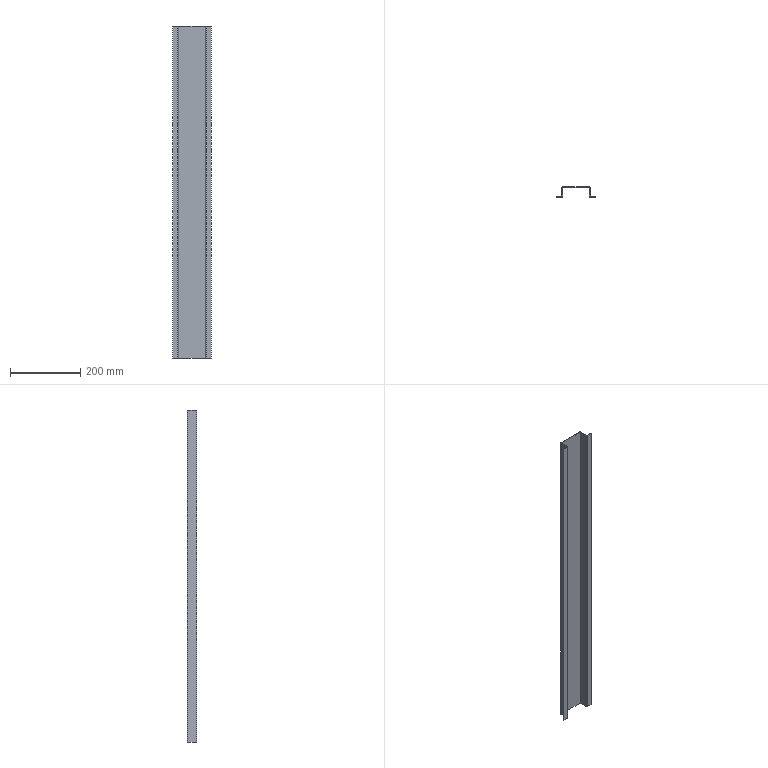Part | SolidWorks | features FlatPattern 1, SMBaseFlange 1, SheetMetal 1 | 1 solid | 38 faces | box 110 x 28.5 x 948 mm | volume 230156 mm3 | plane 30 | cylinder 8 | commonest cylinder face diameters 1 x4 4 x4
STEP:
#1=CARTESIAN_POINT('',(-40.,0.5,474.));
#2=VERTEX_POINT('',#1);
#3=CARTESIAN_POINT('',(-38.5,0.5,474.));
#4=VERTEX_POINT('',#3);
#5=CARTESIAN_POINT('',(-40.,0.5,474.));
#6=DIRECTION('',(1.,0.,0.));
#7=VECTOR('',#6,1000.);
#8=LINE('',#5,#7);
#9=EDGE_CURVE('',#2,#4,#8,.T.);
#10=ORIENTED_EDGE('',*,*,#9,.F.);
#11=CARTESIAN_POINT('',(-40.5,0.,474.));
#12=VERTEX_POINT('',#11);
#13=CARTESIAN_POINT('',(-40.5,0.5,474.));
#14=DIRECTION('',(0.,0.,-1.));
#15=DIRECTION('',(-1.,0.,0.));
#16=AXIS2_PLACEMENT_3D('',#13,#14,#15);
#17=CIRCLE('',#16,0.5);
#18=EDGE_CURVE('',#2,#12,#17,.T.);
#19=ORIENTED_EDGE('',*,*,#18,.T.);
#20=CARTESIAN_POINT('',(-40.5,-1.5,474.));
#21=VERTEX_POINT('',#20);
#22=CARTESIAN_POINT('',(-40.5,-1.5,474.));
#23=DIRECTION('',(0.,1.,0.));
#24=VECTOR('',#23,1000.);
#25=LINE('',#22,#24);
#26=EDGE_CURVE('',#21,#12,#25,.T.);
#27=ORIENTED_EDGE('',*,*,#26,.F.);
#28=CARTESIAN_POINT('',(-40.5,0.5,474.));
#29=DIRECTION('',(0.,0.,-1.));
#30=DIRECTION('',(1.,0.,0.));
#31=AXIS2_PLACEMENT_3D('',#28,#29,#30);
#32=CIRCLE('',#31,2.);
#33=EDGE_CURVE('',#4,#21,#32,.T.);
#34=ORIENTED_EDGE('',*,*,#33,.F.);
#35=EDGE_LOOP('',(#10,#19,#27,#34));
#36=FACE_OUTER_BOUND('',#35,.T.);
#37=CARTESIAN_POINT('',(-40.,0.5,474.));
#38=DIRECTION('',(0.,0.,1.));
#39=DIRECTION('',(1.,0.,0.));
#40=AXIS2_PLACEMENT_3D('',#37,#38,#39);
#41=PLANE('',#40);
#42=ADVANCED_FACE('',(#36),#41,.T.);
#43=CARTESIAN_POINT('',(-40.,25.,474.));
#44=VERTEX_POINT('',#43);
#45=CARTESIAN_POINT('',(-40.,0.,474.));
#46=DIRECTION('',(0.,-1.,0.));
#47=VECTOR('',#46,1000.);
#48=LINE('',#45,#47);
#49=EDGE_CURVE('',#44,#2,#48,.T.);
#50=ORIENTED_EDGE('',*,*,#49,.T.);
#51=ORIENTED_EDGE('',*,*,#9,.T.);
#52=CARTESIAN_POINT('',(-38.5,25.,474.));
#53=VERTEX_POINT('',#52);
#54=CARTESIAN_POINT('',(-38.5,0.,474.));
#55=DIRECTION('',(0.,-1.,0.));
#56=VECTOR('',#55,1000.);
#57=LINE('',#54,#56);
#58=EDGE_CURVE('',#53,#4,#57,.T.);
#59=ORIENTED_EDGE('',*,*,#58,.F.);
#60=CARTESIAN_POINT('',(-38.5,25.,474.));
#61=DIRECTION('',(-1.,0.,0.));
#62=VECTOR('',#61,1000.);
#63=LINE('',#60,#62);
#64=EDGE_CURVE('',#53,#44,#63,.T.);
#65=ORIENTED_EDGE('',*,*,#64,.T.);
#66=EDGE_LOOP('',(#50,#51,#59,#65));
#67=FACE_OUTER_BOUND('',#66,.T.);
#68=CARTESIAN_POINT('',(-40.5,-1.5,474.));
#69=DIRECTION('',(0.,0.,1.));
#70=DIRECTION('',(1.,0.,0.));
#71=AXIS2_PLACEMENT_3D('',#68,#69,#70);
#72=PLANE('',#71);
#73=ADVANCED_FACE('',(#67),#72,.T.);
#74=CARTESIAN_POINT('',(-40.5,0.,-474.));
#75=VERTEX_POINT('',#74);
#76=CARTESIAN_POINT('',(-40.5,-1.5,-474.));
#77=VERTEX_POINT('',#76);
#78=CARTESIAN_POINT('',(-40.5,0.,-474.));
#79=DIRECTION('',(0.,-1.,0.));
#80=VECTOR('',#79,1000.);
#81=LINE('',#78,#80);
#82=EDGE_CURVE('',#75,#77,#81,.T.);
#83=ORIENTED_EDGE('',*,*,#82,.F.);
#84=CARTESIAN_POINT('',(-40.,0.5,-474.));
#85=VERTEX_POINT('',#84);
#86=CARTESIAN_POINT('',(-40.5,0.5,-474.));
#87=DIRECTION('',(0.,0.,-1.));
#88=DIRECTION('',(-1.,0.,0.));
#89=AXIS2_PLACEMENT_3D('',#86,#87,#88);
#90=CIRCLE('',#89,0.5);
#91=EDGE_CURVE('',#85,#75,#90,.T.);
#92=ORIENTED_EDGE('',*,*,#91,.F.);
#93=CARTESIAN_POINT('',(-38.5,0.5,-474.));
#94=VERTEX_POINT('',#93);
#95=CARTESIAN_POINT('',(-38.5,0.5,-474.));
#96=DIRECTION('',(-1.,0.,0.));
#97=VECTOR('',#96,1000.);
#98=LINE('',#95,#97);
#99=EDGE_CURVE('',#94,#85,#98,.T.);
#100=ORIENTED_EDGE('',*,*,#99,.F.);
#101=CARTESIAN_POINT('',(-40.5,0.5,-474.));
#102=DIRECTION('',(0.,0.,-1.));
#103=DIRECTION('',(1.,0.,0.));
#104=AXIS2_PLACEMENT_3D('',#101,#102,#103);
#105=CIRCLE('',#104,2.);
#106=EDGE_CURVE('',#94,#77,#105,.T.);
#107=ORIENTED_EDGE('',*,*,#106,.T.);
#108=EDGE_LOOP('',(#83,#92,#100,#107));
#109=FACE_OUTER_BOUND('',#108,.T.);
#110=CARTESIAN_POINT('',(-40.5,0.,-474.));
#111=DIRECTION('',(0.,0.,-1.));
#112=DIRECTION('',(-1.,0.,0.));
#113=AXIS2_PLACEMENT_3D('',#110,#111,#112);
#114=PLANE('',#113);
#115=ADVANCED_FACE('',(#109),#114,.T.);
#116=CARTESIAN_POINT('',(-55.,0.,-474.));
#117=VERTEX_POINT('',#116);
#118=CARTESIAN_POINT('',(-55.,0.,-474.));
#119=DIRECTION('',(-1.,0.,0.));
#120=VECTOR('',#119,1000.);
#121=LINE('',#118,#120);
#122=EDGE_CURVE('',#75,#117,#121,.T.);
#123=ORIENTED_EDGE('',*,*,#122,.F.);
#124=ORIENTED_EDGE('',*,*,#82,.T.);
#125=CARTESIAN_POINT('',(-55.,-1.5,-474.));
#126=VERTEX_POINT('',#125);
#127=CARTESIAN_POINT('',(-55.,-1.5,-474.));
#128=DIRECTION('',(-1.,0.,0.));
#129=VECTOR('',#128,1000.);
#130=LINE('',#127,#129);
#131=EDGE_CURVE('',#77,#126,#130,.T.);
#132=ORIENTED_EDGE('',*,*,#131,.T.);
#133=CARTESIAN_POINT('',(-55.,-1.5,-474.));
#134=DIRECTION('',(0.,1.,0.));
#135=VECTOR('',#134,1000.);
#136=LINE('',#133,#135);
#137=EDGE_CURVE('',#126,#117,#136,.T.);
#138=ORIENTED_EDGE('',*,*,#137,.T.);
#139=EDGE_LOOP('',(#123,#124,#132,#138));
#140=FACE_OUTER_BOUND('',#139,.T.);
#141=CARTESIAN_POINT('',(-38.5,0.5,-474.));
#142=DIRECTION('',(0.,0.,-1.));
#143=DIRECTION('',(-1.,0.,0.));
#144=AXIS2_PLACEMENT_3D('',#141,#142,#143);
#145=PLANE('',#144);
#146=ADVANCED_FACE('',(#140),#145,.T.);
#147=CARTESIAN_POINT('',(-38.,27.,474.));
#148=VERTEX_POINT('',#147);
#149=CARTESIAN_POINT('',(-38.,25.5,474.));
#150=VERTEX_POINT('',#149);
#151=CARTESIAN_POINT('',(-38.,27.,474.));
#152=DIRECTION('',(0.,-1.,0.));
#153=VECTOR('',#152,1000.);
#154=LINE('',#151,#153);
#155=EDGE_CURVE('',#148,#150,#154,.T.);
#156=ORIENTED_EDGE('',*,*,#155,.F.);
#157=CARTESIAN_POINT('',(-38.,25.,474.));
#158=DIRECTION('',(0.,0.,1.));
#159=DIRECTION('',(1.,0.,0.));
#160=AXIS2_PLACEMENT_3D('',#157,#158,#159);
#161=CIRCLE('',#160,2.);
#162=EDGE_CURVE('',#148,#44,#161,.T.);
#163=ORIENTED_EDGE('',*,*,#162,.T.);
#164=ORIENTED_EDGE('',*,*,#64,.F.);
#165=CARTESIAN_POINT('',(-38.,25.,474.));
#166=DIRECTION('',(0.,0.,1.));
#167=DIRECTION('',(1.,0.,0.));
#168=AXIS2_PLACEMENT_3D('',#165,#166,#167);
#169=CIRCLE('',#168,0.5);
#170=EDGE_CURVE('',#150,#53,#169,.T.);
#171=ORIENTED_EDGE('',*,*,#170,.F.);
#172=EDGE_LOOP('',(#156,#163,#164,#171));
#173=FACE_OUTER_BOUND('',#172,.T.);
#174=CARTESIAN_POINT('',(-38.,27.,474.));
#175=DIRECTION('',(0.,0.,1.));
#176=DIRECTION('',(1.,0.,0.));
#177=AXIS2_PLACEMENT_3D('',#174,#175,#176);
#178=PLANE('',#177);
#179=ADVANCED_FACE('',(#173),#178,.T.);
#180=CARTESIAN_POINT('',(38.,27.,474.));
#181=VERTEX_POINT('',#180);
#182=CARTESIAN_POINT('',(-40.,27.,474.));
#183=DIRECTION('',(-1.,0.,0.));
#184=VECTOR('',#183,1000.);
#185=LINE('',#182,#184);
#186=EDGE_CURVE('',#181,#148,#185,.T.);
#187=ORIENTED_EDGE('',*,*,#186,.T.);
#188=ORIENTED_EDGE('',*,*,#155,.T.);
#189=CARTESIAN_POINT('',(38.,25.5,474.));
#190=VERTEX_POINT('',#189);
#191=CARTESIAN_POINT('',(-40.,25.5,474.));
#192=DIRECTION('',(-1.,0.,0.));
#193=VECTOR('',#192,1000.);
#194=LINE('',#191,#193);
#195=EDGE_CURVE('',#190,#150,#194,.T.);
#196=ORIENTED_EDGE('',*,*,#195,.F.);
#197=CARTESIAN_POINT('',(38.,25.5,474.));
#198=DIRECTION('',(0.,1.,0.));
#199=VECTOR('',#198,1000.);
#200=LINE('',#197,#199);
#201=EDGE_CURVE('',#190,#181,#200,.T.);
#202=ORIENTED_EDGE('',*,*,#201,.T.);
#203=EDGE_LOOP('',(#187,#188,#196,#202));
#204=FACE_OUTER_BOUND('',#203,.T.);
#205=CARTESIAN_POINT('',(-38.5,25.,474.));
#206=DIRECTION('',(0.,0.,1.));
#207=DIRECTION('',(1.,0.,0.));
#208=AXIS2_PLACEMENT_3D('',#205,#206,#207);
#209=PLANE('',#208);
#210=ADVANCED_FACE('',(#204),#209,.T.);
#211=CARTESIAN_POINT('',(-40.,25.,-474.));
#212=VERTEX_POINT('',#211);
#213=CARTESIAN_POINT('',(-38.5,25.,-474.));
#214=VERTEX_POINT('',#213);
#215=CARTESIAN_POINT('',(-40.,25.,-474.));
#216=DIRECTION('',(1.,0.,0.));
#217=VECTOR('',#216,1000.);
#218=LINE('',#215,#217);
#219=EDGE_CURVE('',#212,#214,#218,.T.);
#220=ORIENTED_EDGE('',*,*,#219,.F.);
#221=CARTESIAN_POINT('',(-38.,27.,-474.));
#222=VERTEX_POINT('',#221);
#223=CARTESIAN_POINT('',(-38.,25.,-474.));
#224=DIRECTION('',(0.,0.,1.));
#225=DIRECTION('',(1.,0.,0.));
#226=AXIS2_PLACEMENT_3D('',#223,#224,#225);
#227=CIRCLE('',#226,2.);
#228=EDGE_CURVE('',#222,#212,#227,.T.);
#229=ORIENTED_EDGE('',*,*,#228,.F.);
#230=CARTESIAN_POINT('',(-38.,25.5,-474.));
#231=VERTEX_POINT('',#230);
#232=CARTESIAN_POINT('',(-38.,25.5,-474.));
#233=DIRECTION('',(0.,1.,0.));
#234=VECTOR('',#233,1000.);
#235=LINE('',#232,#234);
#236=EDGE_CURVE('',#231,#222,#235,.T.);
#237=ORIENTED_EDGE('',*,*,#236,.F.);
#238=CARTESIAN_POINT('',(-38.,25.,-474.));
#239=DIRECTION('',(0.,0.,1.));
#240=DIRECTION('',(1.,0.,0.));
#241=AXIS2_PLACEMENT_3D('',#238,#239,#240);
#242=CIRCLE('',#241,0.5);
#243=EDGE_CURVE('',#231,#214,#242,.T.);
#244=ORIENTED_EDGE('',*,*,#243,.T.);
#245=EDGE_LOOP('',(#220,#229,#237,#244));
#246=FACE_OUTER_BOUND('',#245,.T.);
#247=CARTESIAN_POINT('',(-40.,25.,-474.));
#248=DIRECTION('',(0.,0.,-1.));
#249=DIRECTION('',(-1.,0.,0.));
#250=AXIS2_PLACEMENT_3D('',#247,#248,#249);
#251=PLANE('',#250);
#252=ADVANCED_FACE('',(#246),#251,.T.);
#253=CARTESIAN_POINT('',(-40.,0.,-474.));
#254=DIRECTION('',(0.,-1.,0.));
#255=VECTOR('',#254,1000.);
#256=LINE('',#253,#255);
#257=EDGE_CURVE('',#212,#85,#256,.T.);
#258=ORIENTED_EDGE('',*,*,#257,.F.);
#259=ORIENTED_EDGE('',*,*,#219,.T.);
#260=CARTESIAN_POINT('',(-38.5,0.,-474.));
#261=DIRECTION('',(0.,-1.,0.));
#262=VECTOR('',#261,1000.);
#263=LINE('',#260,#262);
#264=EDGE_CURVE('',#214,#94,#263,.T.);
#265=ORIENTED_EDGE('',*,*,#264,.T.);
#266=ORIENTED_EDGE('',*,*,#99,.T.);
#267=EDGE_LOOP('',(#258,#259,#265,#266));
#268=FACE_OUTER_BOUND('',#267,.T.);
#269=CARTESIAN_POINT('',(-38.,25.5,-474.));
#270=DIRECTION('',(0.,0.,-1.));
#271=DIRECTION('',(-1.,0.,0.));
#272=AXIS2_PLACEMENT_3D('',#269,#270,#271);
#273=PLANE('',#272);
#274=ADVANCED_FACE('',(#268),#273,.T.);
#275=CARTESIAN_POINT('',(40.,25.,474.));
#276=VERTEX_POINT('',#275);
#277=CARTESIAN_POINT('',(38.5,25.,474.));
#278=VERTEX_POINT('',#277);
#279=CARTESIAN_POINT('',(40.,25.,474.));
#280=DIRECTION('',(-1.,0.,0.));
#281=VECTOR('',#280,1000.);
#282=LINE('',#279,#281);
#283=EDGE_CURVE('',#276,#278,#282,.T.);
#284=ORIENTED_EDGE('',*,*,#283,.F.);
#285=CARTESIAN_POINT('',(38.,25.,474.));
#286=DIRECTION('',(0.,0.,1.));
#287=DIRECTION('',(1.,0.,0.));
#288=AXIS2_PLACEMENT_3D('',#285,#286,#287);
#289=CIRCLE('',#288,2.);
#290=EDGE_CURVE('',#276,#181,#289,.T.);
#291=ORIENTED_EDGE('',*,*,#290,.T.);
#292=ORIENTED_EDGE('',*,*,#201,.F.);
#293=CARTESIAN_POINT('',(38.,25.,474.));
#294=DIRECTION('',(0.,0.,1.));
#295=DIRECTION('',(1.,0.,0.));
#296=AXIS2_PLACEMENT_3D('',#293,#294,#295);
#297=CIRCLE('',#296,0.5);
#298=EDGE_CURVE('',#278,#190,#297,.T.);
#299=ORIENTED_EDGE('',*,*,#298,.F.);
#300=EDGE_LOOP('',(#284,#291,#292,#299));
#301=FACE_OUTER_BOUND('',#300,.T.);
#302=CARTESIAN_POINT('',(40.,25.,474.));
#303=DIRECTION('',(0.,0.,1.));
#304=DIRECTION('',(1.,0.,0.));
#305=AXIS2_PLACEMENT_3D('',#302,#303,#304);
#306=PLANE('',#305);
#307=ADVANCED_FACE('',(#301),#306,.T.);
#308=CARTESIAN_POINT('',(40.,0.5,474.));
#309=VERTEX_POINT('',#308);
#310=CARTESIAN_POINT('',(40.,0.,474.));
#311=DIRECTION('',(0.,1.,0.));
#312=VECTOR('',#311,1000.);
#313=LINE('',#310,#312);
#314=EDGE_CURVE('',#309,#276,#313,.T.);
#315=ORIENTED_EDGE('',*,*,#314,.T.);
#316=ORIENTED_EDGE('',*,*,#283,.T.);
#317=CARTESIAN_POINT('',(38.5,0.5,474.));
#318=VERTEX_POINT('',#317);
#319=CARTESIAN_POINT('',(38.5,0.,474.));
#320=DIRECTION('',(0.,1.,0.));
#321=VECTOR('',#320,1000.);
#322=LINE('',#319,#321);
#323=EDGE_CURVE('',#318,#278,#322,.T.);
#324=ORIENTED_EDGE('',*,*,#323,.F.);
#325=CARTESIAN_POINT('',(38.5,0.5,474.));
#326=DIRECTION('',(1.,0.,0.));
#327=VECTOR('',#326,1000.);
#328=LINE('',#325,#327);
#329=EDGE_CURVE('',#318,#309,#328,.T.);
#330=ORIENTED_EDGE('',*,*,#329,.T.);
#331=EDGE_LOOP('',(#315,#316,#324,#330));
#332=FACE_OUTER_BOUND('',#331,.T.);
#333=CARTESIAN_POINT('',(38.,25.5,474.));
#334=DIRECTION('',(0.,0.,1.));
#335=DIRECTION('',(1.,0.,0.));
#336=AXIS2_PLACEMENT_3D('',#333,#334,#335);
#337=PLANE('',#336);
#338=ADVANCED_FACE('',(#332),#337,.T.);
#339=CARTESIAN_POINT('',(38.,27.,-474.));
#340=VERTEX_POINT('',#339);
#341=CARTESIAN_POINT('',(38.,25.5,-474.));
#342=VERTEX_POINT('',#341);
#343=CARTESIAN_POINT('',(38.,27.,-474.));
#344=DIRECTION('',(0.,-1.,0.));
#345=VECTOR('',#344,1000.);
#346=LINE('',#343,#345);
#347=EDGE_CURVE('',#340,#342,#346,.T.);
#348=ORIENTED_EDGE('',*,*,#347,.F.);
#349=CARTESIAN_POINT('',(40.,25.,-474.));
#350=VERTEX_POINT('',#349);
#351=CARTESIAN_POINT('',(38.,25.,-474.));
#352=DIRECTION('',(0.,0.,1.));
#353=DIRECTION('',(1.,0.,0.));
#354=AXIS2_PLACEMENT_3D('',#351,#352,#353);
#355=CIRCLE('',#354,2.);
#356=EDGE_CURVE('',#350,#340,#355,.T.);
#357=ORIENTED_EDGE('',*,*,#356,.F.);
#358=CARTESIAN_POINT('',(38.5,25.,-474.));
#359=VERTEX_POINT('',#358);
#360=CARTESIAN_POINT('',(38.5,25.,-474.));
#361=DIRECTION('',(1.,0.,0.));
#362=VECTOR('',#361,1000.);
#363=LINE('',#360,#362);
#364=EDGE_CURVE('',#359,#350,#363,.T.);
#365=ORIENTED_EDGE('',*,*,#364,.F.);
#366=CARTESIAN_POINT('',(38.,25.,-474.));
#367=DIRECTION('',(0.,0.,1.));
#368=DIRECTION('',(1.,0.,0.));
#369=AXIS2_PLACEMENT_3D('',#366,#367,#368);
#370=CIRCLE('',#369,0.5);
#371=EDGE_CURVE('',#359,#342,#370,.T.);
#372=ORIENTED_EDGE('',*,*,#371,.T.);
#373=EDGE_LOOP('',(#348,#357,#365,#372));
#374=FACE_OUTER_BOUND('',#373,.T.);
#375=CARTESIAN_POINT('',(38.,27.,-474.));
#376=DIRECTION('',(0.,0.,-1.));
#377=DIRECTION('',(-1.,0.,0.));
#378=AXIS2_PLACEMENT_3D('',#375,#376,#377);
#379=PLANE('',#378);
#380=ADVANCED_FACE('',(#374),#379,.T.);
#381=CARTESIAN_POINT('',(-40.,27.,-474.));
#382=DIRECTION('',(-1.,0.,0.));
#383=VECTOR('',#382,1000.);
#384=LINE('',#381,#383);
#385=EDGE_CURVE('',#340,#222,#384,.T.);
#386=ORIENTED_EDGE('',*,*,#385,.F.);
#387=ORIENTED_EDGE('',*,*,#347,.T.);
#388=CARTESIAN_POINT('',(-40.,25.5,-474.));
#389=DIRECTION('',(-1.,0.,0.));
#390=VECTOR('',#389,1000.);
#391=LINE('',#388,#390);
#392=EDGE_CURVE('',#342,#231,#391,.T.);
#393=ORIENTED_EDGE('',*,*,#392,.T.);
#394=ORIENTED_EDGE('',*,*,#236,.T.);
#395=EDGE_LOOP('',(#386,#387,#393,#394));
#396=FACE_OUTER_BOUND('',#395,.T.);
#397=CARTESIAN_POINT('',(38.5,25.,-474.));
#398=DIRECTION('',(0.,0.,-1.));
#399=DIRECTION('',(-1.,0.,0.));
#400=AXIS2_PLACEMENT_3D('',#397,#398,#399);
#401=PLANE('',#400);
#402=ADVANCED_FACE('',(#396),#401,.T.);
#403=CARTESIAN_POINT('',(40.5,0.,474.));
#404=VERTEX_POINT('',#403);
#405=CARTESIAN_POINT('',(40.5,-1.5,474.));
#406=VERTEX_POINT('',#405);
#407=CARTESIAN_POINT('',(40.5,0.,474.));
#408=DIRECTION('',(0.,-1.,0.));
#409=VECTOR('',#408,1000.);
#410=LINE('',#407,#409);
#411=EDGE_CURVE('',#404,#406,#410,.T.);
#412=ORIENTED_EDGE('',*,*,#411,.F.);
#413=CARTESIAN_POINT('',(40.5,0.5,474.));
#414=DIRECTION('',(0.,0.,-1.));
#415=DIRECTION('',(-1.,0.,0.));
#416=AXIS2_PLACEMENT_3D('',#413,#414,#415);
#417=CIRCLE('',#416,0.5);
#418=EDGE_CURVE('',#404,#309,#417,.T.);
#419=ORIENTED_EDGE('',*,*,#418,.T.);
#420=ORIENTED_EDGE('',*,*,#329,.F.);
#421=CARTESIAN_POINT('',(40.5,0.5,474.));
#422=DIRECTION('',(0.,0.,-1.));
#423=DIRECTION('',(1.,0.,0.));
#424=AXIS2_PLACEMENT_3D('',#421,#422,#423);
#425=CIRCLE('',#424,2.);
#426=EDGE_CURVE('',#406,#318,#425,.T.);
#427=ORIENTED_EDGE('',*,*,#426,.F.);
#428=EDGE_LOOP('',(#412,#419,#420,#427));
#429=FACE_OUTER_BOUND('',#428,.T.);
#430=CARTESIAN_POINT('',(40.5,0.,474.));
#431=DIRECTION('',(0.,0.,1.));
#432=DIRECTION('',(1.,0.,0.));
#433=AXIS2_PLACEMENT_3D('',#430,#431,#432);
#434=PLANE('',#433);
#435=ADVANCED_FACE('',(#429),#434,.T.);
#436=CARTESIAN_POINT('',(55.,0.,474.));
#437=VERTEX_POINT('',#436);
#438=CARTESIAN_POINT('',(55.,0.,474.));
#439=DIRECTION('',(-1.,0.,0.));
#440=VECTOR('',#439,1000.);
#441=LINE('',#438,#440);
#442=EDGE_CURVE('',#437,#404,#441,.T.);
#443=ORIENTED_EDGE('',*,*,#442,.T.);
#444=ORIENTED_EDGE('',*,*,#411,.T.);
#445=CARTESIAN_POINT('',(55.,-1.5,474.));
#446=VERTEX_POINT('',#445);
#447=CARTESIAN_POINT('',(55.,-1.5,474.));
#448=DIRECTION('',(-1.,0.,0.));
#449=VECTOR('',#448,1000.);
#450=LINE('',#447,#449);
#451=EDGE_CURVE('',#446,#406,#450,.T.);
#452=ORIENTED_EDGE('',*,*,#451,.F.);
#453=CARTESIAN_POINT('',(55.,0.,474.));
#454=DIRECTION('',(0.,-1.,0.));
#455=VECTOR('',#454,1000.);
#456=LINE('',#453,#455);
#457=EDGE_CURVE('',#437,#446,#456,.T.);
#458=ORIENTED_EDGE('',*,*,#457,.F.);
#459=EDGE_LOOP('',(#443,#444,#452,#458));
#460=FACE_OUTER_BOUND('',#459,.T.);
#461=CARTESIAN_POINT('',(38.5,0.5,474.));
#462=DIRECTION('',(0.,0.,1.));
#463=DIRECTION('',(1.,0.,0.));
#464=AXIS2_PLACEMENT_3D('',#461,#462,#463);
#465=PLANE('',#464);
#466=ADVANCED_FACE('',(#460),#465,.T.);
#467=CARTESIAN_POINT('',(40.,0.5,-474.));
#468=VERTEX_POINT('',#467);
#469=CARTESIAN_POINT('',(38.5,0.5,-474.));
#470=VERTEX_POINT('',#469);
#471=CARTESIAN_POINT('',(40.,0.5,-474.));
#472=DIRECTION('',(-1.,0.,0.));
#473=VECTOR('',#472,1000.);
#474=LINE('',#471,#473);
#475=EDGE_CURVE('',#468,#470,#474,.T.);
#476=ORIENTED_EDGE('',*,*,#475,.F.);
#477=CARTESIAN_POINT('',(40.5,0.,-474.));
#478=VERTEX_POINT('',#477);
#479=CARTESIAN_POINT('',(40.5,0.5,-474.));
#480=DIRECTION('',(0.,0.,-1.));
#481=DIRECTION('',(-1.,0.,0.));
#482=AXIS2_PLACEMENT_3D('',#479,#480,#481);
#483=CIRCLE('',#482,0.5);
#484=EDGE_CURVE('',#478,#468,#483,.T.);
#485=ORIENTED_EDGE('',*,*,#484,.F.);
#486=CARTESIAN_POINT('',(40.5,-1.5,-474.));
#487=VERTEX_POINT('',#486);
#488=CARTESIAN_POINT('',(40.5,-1.5,-474.));
#489=DIRECTION('',(0.,1.,0.));
#490=VECTOR('',#489,1000.);
#491=LINE('',#488,#490);
#492=EDGE_CURVE('',#487,#478,#491,.T.);
#493=ORIENTED_EDGE('',*,*,#492,.F.);
#494=CARTESIAN_POINT('',(40.5,0.5,-474.));
#495=DIRECTION('',(0.,0.,-1.));
#496=DIRECTION('',(1.,0.,0.));
#497=AXIS2_PLACEMENT_3D('',#494,#495,#496);
#498=CIRCLE('',#497,2.);
#499=EDGE_CURVE('',#487,#470,#498,.T.);
#500=ORIENTED_EDGE('',*,*,#499,.T.);
#501=EDGE_LOOP('',(#476,#485,#493,#500));
#502=FACE_OUTER_BOUND('',#501,.T.);
#503=CARTESIAN_POINT('',(40.,0.5,-474.));
#504=DIRECTION('',(0.,0.,-1.));
#505=DIRECTION('',(-1.,0.,0.));
#506=AXIS2_PLACEMENT_3D('',#503,#504,#505);
#507=PLANE('',#506);
#508=ADVANCED_FACE('',(#502),#507,.T.);
#509=CARTESIAN_POINT('',(40.,0.,-474.));
#510=DIRECTION('',(0.,1.,0.));
#511=VECTOR('',#510,1000.);
#512=LINE('',#509,#511);
#513=EDGE_CURVE('',#468,#350,#512,.T.);
#514=ORIENTED_EDGE('',*,*,#513,.F.);
#515=ORIENTED_EDGE('',*,*,#475,.T.);
#516=CARTESIAN_POINT('',(38.5,0.,-474.));
#517=DIRECTION('',(0.,1.,0.));
#518=VECTOR('',#517,1000.);
#519=LINE('',#516,#518);
#520=EDGE_CURVE('',#470,#359,#519,.T.);
#521=ORIENTED_EDGE('',*,*,#520,.T.);
#522=ORIENTED_EDGE('',*,*,#364,.T.);
#523=EDGE_LOOP('',(#514,#515,#521,#522));
#524=FACE_OUTER_BOUND('',#523,.T.);
#525=CARTESIAN_POINT('',(40.5,-1.5,-474.));
#526=DIRECTION('',(0.,0.,-1.));
#527=DIRECTION('',(-1.,0.,0.));
#528=AXIS2_PLACEMENT_3D('',#525,#526,#527);
#529=PLANE('',#528);
#530=ADVANCED_FACE('',(#524),#529,.T.);
#531=ORIENTED_EDGE('',*,*,#122,.T.);
#532=CARTESIAN_POINT('',(-55.,0.,474.));
#533=VERTEX_POINT('',#532);
#534=CARTESIAN_POINT('',(-55.,0.,474.));
#535=DIRECTION('',(0.,0.,-1.));
#536=VECTOR('',#535,1000.);
#537=LINE('',#534,#536);
#538=EDGE_CURVE('',#533,#117,#537,.T.);
#539=ORIENTED_EDGE('',*,*,#538,.F.);
#540=CARTESIAN_POINT('',(-55.,0.,474.));
#541=DIRECTION('',(-1.,0.,0.));
#542=VECTOR('',#541,1000.);
#543=LINE('',#540,#542);
#544=EDGE_CURVE('',#12,#533,#543,.T.);
#545=ORIENTED_EDGE('',*,*,#544,.F.);
#546=CARTESIAN_POINT('',(-40.5,0.,474.));
#547=DIRECTION('',(0.,0.,-1.));
#548=VECTOR('',#547,1000.);
#549=LINE('',#546,#548);
#550=EDGE_CURVE('',#12,#75,#549,.T.);
#551=ORIENTED_EDGE('',*,*,#550,.T.);
#552=EDGE_LOOP('',(#531,#539,#545,#551));
#553=FACE_OUTER_BOUND('',#552,.T.);
#554=CARTESIAN_POINT('',(-55.,0.,474.));
#555=DIRECTION('',(0.,-1.,0.));
#556=DIRECTION('',(0.,0.,-1.));
#557=AXIS2_PLACEMENT_3D('',#554,#555,#556);
#558=PLANE('',#557);
#559=ADVANCED_FACE('',(#553),#558,.F.);
#560=ORIENTED_EDGE('',*,*,#137,.F.);
#561=CARTESIAN_POINT('',(-55.,-1.5,474.));
#562=VERTEX_POINT('',#561);
#563=CARTESIAN_POINT('',(-55.,-1.5,474.));
#564=DIRECTION('',(0.,0.,-1.));
#565=VECTOR('',#564,1000.);
#566=LINE('',#563,#565);
#567=EDGE_CURVE('',#562,#126,#566,.T.);
#568=ORIENTED_EDGE('',*,*,#567,.F.);
#569=CARTESIAN_POINT('',(-55.,-1.5,474.));
#570=DIRECTION('',(0.,1.,0.));
#571=VECTOR('',#570,1000.);
#572=LINE('',#569,#571);
#573=EDGE_CURVE('',#562,#533,#572,.T.);
#574=ORIENTED_EDGE('',*,*,#573,.T.);
#575=ORIENTED_EDGE('',*,*,#538,.T.);
#576=EDGE_LOOP('',(#560,#568,#574,#575));
#577=FACE_OUTER_BOUND('',#576,.T.);
#578=CARTESIAN_POINT('',(-55.,-1.5,474.));
#579=DIRECTION('',(-1.,0.,0.));
#580=DIRECTION('',(0.,0.,1.));
#581=AXIS2_PLACEMENT_3D('',#578,#579,#580);
#582=PLANE('',#581);
#583=ADVANCED_FACE('',(#577),#582,.T.);
#584=ORIENTED_EDGE('',*,*,#131,.F.);
#585=CARTESIAN_POINT('',(-40.5,-1.5,474.));
#586=DIRECTION('',(0.,0.,-1.));
#587=VECTOR('',#586,1000.);
#588=LINE('',#585,#587);
#589=EDGE_CURVE('',#21,#77,#588,.T.);
#590=ORIENTED_EDGE('',*,*,#589,.F.);
#591=CARTESIAN_POINT('',(-55.,-1.5,474.));
#592=DIRECTION('',(-1.,0.,0.));
#593=VECTOR('',#592,1000.);
#594=LINE('',#591,#593);
#595=EDGE_CURVE('',#21,#562,#594,.T.);
#596=ORIENTED_EDGE('',*,*,#595,.T.);
#597=ORIENTED_EDGE('',*,*,#567,.T.);
#598=EDGE_LOOP('',(#584,#590,#596,#597));
#599=FACE_OUTER_BOUND('',#598,.T.);
#600=CARTESIAN_POINT('',(-55.,-1.5,474.));
#601=DIRECTION('',(0.,-1.,0.));
#602=DIRECTION('',(0.,0.,-1.));
#603=AXIS2_PLACEMENT_3D('',#600,#601,#602);
#604=PLANE('',#603);
#605=ADVANCED_FACE('',(#599),#604,.T.);
#606=ORIENTED_EDGE('',*,*,#106,.F.);
#607=CARTESIAN_POINT('',(-38.5,0.5,474.));
#608=DIRECTION('',(0.,0.,-1.));
#609=VECTOR('',#608,1000.);
#610=LINE('',#607,#609);
#611=EDGE_CURVE('',#4,#94,#610,.T.);
#612=ORIENTED_EDGE('',*,*,#611,.F.);
#613=ORIENTED_EDGE('',*,*,#33,.T.);
#614=ORIENTED_EDGE('',*,*,#589,.T.);
#615=EDGE_LOOP('',(#606,#612,#613,#614));
#616=FACE_OUTER_BOUND('',#615,.T.);
#617=CARTESIAN_POINT('',(-40.5,0.5,474.));
#618=DIRECTION('',(0.,0.,-1.));
#619=DIRECTION('',(-1.,0.,0.));
#620=AXIS2_PLACEMENT_3D('',#617,#618,#619);
#621=CYLINDRICAL_SURFACE('',#620,2.);
#622=ADVANCED_FACE('',(#616),#621,.T.);
#623=ORIENTED_EDGE('',*,*,#264,.F.);
#624=CARTESIAN_POINT('',(-38.5,25.,474.));
#625=DIRECTION('',(0.,0.,-1.));
#626=VECTOR('',#625,1000.);
#627=LINE('',#624,#626);
#628=EDGE_CURVE('',#53,#214,#627,.T.);
#629=ORIENTED_EDGE('',*,*,#628,.F.);
#630=ORIENTED_EDGE('',*,*,#58,.T.);
#631=ORIENTED_EDGE('',*,*,#611,.T.);
#632=EDGE_LOOP('',(#623,#629,#630,#631));
#633=FACE_OUTER_BOUND('',#632,.T.);
#634=CARTESIAN_POINT('',(-38.5,0.,474.));
#635=DIRECTION('',(1.,0.,0.));
#636=DIRECTION('',(0.,1.,0.));
#637=AXIS2_PLACEMENT_3D('',#634,#635,#636);
#638=PLANE('',#637);
#639=ADVANCED_FACE('',(#633),#638,.T.);
#640=ORIENTED_EDGE('',*,*,#243,.F.);
#641=CARTESIAN_POINT('',(-38.,25.5,474.));
#642=DIRECTION('',(0.,0.,-1.));
#643=VECTOR('',#642,1000.);
#644=LINE('',#641,#643);
#645=EDGE_CURVE('',#150,#231,#644,.T.);
#646=ORIENTED_EDGE('',*,*,#645,.F.);
#647=ORIENTED_EDGE('',*,*,#170,.T.);
#648=ORIENTED_EDGE('',*,*,#628,.T.);
#649=EDGE_LOOP('',(#640,#646,#647,#648));
#650=FACE_OUTER_BOUND('',#649,.T.);
#651=CARTESIAN_POINT('',(-38.,25.,474.));
#652=DIRECTION('',(0.,0.,-1.));
#653=DIRECTION('',(-1.,0.,0.));
#654=AXIS2_PLACEMENT_3D('',#651,#652,#653);
#655=CYLINDRICAL_SURFACE('',#654,0.5);
#656=ADVANCED_FACE('',(#650),#655,.F.);
#657=ORIENTED_EDGE('',*,*,#392,.F.);
#658=CARTESIAN_POINT('',(38.,25.5,474.));
#659=DIRECTION('',(0.,0.,-1.));
#660=VECTOR('',#659,1000.);
#661=LINE('',#658,#660);
#662=EDGE_CURVE('',#190,#342,#661,.T.);
#663=ORIENTED_EDGE('',*,*,#662,.F.);
#664=ORIENTED_EDGE('',*,*,#195,.T.);
#665=ORIENTED_EDGE('',*,*,#645,.T.);
#666=EDGE_LOOP('',(#657,#663,#664,#665));
#667=FACE_OUTER_BOUND('',#666,.T.);
#668=CARTESIAN_POINT('',(-40.,25.5,474.));
#669=DIRECTION('',(0.,-1.,0.));
#670=DIRECTION('',(0.,0.,-1.));
#671=AXIS2_PLACEMENT_3D('',#668,#669,#670);
#672=PLANE('',#671);
#673=ADVANCED_FACE('',(#667),#672,.T.);
#674=ORIENTED_EDGE('',*,*,#371,.F.);
#675=CARTESIAN_POINT('',(38.5,25.,474.));
#676=DIRECTION('',(0.,0.,-1.));
#677=VECTOR('',#676,1000.);
#678=LINE('',#675,#677);
#679=EDGE_CURVE('',#278,#359,#678,.T.);
#680=ORIENTED_EDGE('',*,*,#679,.F.);
#681=ORIENTED_EDGE('',*,*,#298,.T.);
#682=ORIENTED_EDGE('',*,*,#662,.T.);
#683=EDGE_LOOP('',(#674,#680,#681,#682));
#684=FACE_OUTER_BOUND('',#683,.T.);
#685=CARTESIAN_POINT('',(38.,25.,474.));
#686=DIRECTION('',(0.,0.,-1.));
#687=DIRECTION('',(-1.,0.,0.));
#688=AXIS2_PLACEMENT_3D('',#685,#686,#687);
#689=CYLINDRICAL_SURFACE('',#688,0.5);
#690=ADVANCED_FACE('',(#684),#689,.F.);
#691=ORIENTED_EDGE('',*,*,#520,.F.);
#692=CARTESIAN_POINT('',(38.5,0.5,474.));
#693=DIRECTION('',(0.,0.,-1.));
#694=VECTOR('',#693,1000.);
#695=LINE('',#692,#694);
#696=EDGE_CURVE('',#318,#470,#695,.T.);
#697=ORIENTED_EDGE('',*,*,#696,.F.);
#698=ORIENTED_EDGE('',*,*,#323,.T.);
#699=ORIENTED_EDGE('',*,*,#679,.T.);
#700=EDGE_LOOP('',(#691,#697,#698,#699));
#701=FACE_OUTER_BOUND('',#700,.T.);
#702=CARTESIAN_POINT('',(38.5,0.,474.));
#703=DIRECTION('',(-1.,0.,0.));
#704=DIRECTION('',(0.,-1.,0.));
#705=AXIS2_PLACEMENT_3D('',#702,#703,#704);
#706=PLANE('',#705);
#707=ADVANCED_FACE('',(#701),#706,.T.);
#708=ORIENTED_EDGE('',*,*,#499,.F.);
#709=CARTESIAN_POINT('',(40.5,-1.5,474.));
#710=DIRECTION('',(0.,0.,-1.));
#711=VECTOR('',#710,1000.);
#712=LINE('',#709,#711);
#713=EDGE_CURVE('',#406,#487,#712,.T.);
#714=ORIENTED_EDGE('',*,*,#713,.F.);
#715=ORIENTED_EDGE('',*,*,#426,.T.);
#716=ORIENTED_EDGE('',*,*,#696,.T.);
#717=EDGE_LOOP('',(#708,#714,#715,#716));
#718=FACE_OUTER_BOUND('',#717,.T.);
#719=CARTESIAN_POINT('',(40.5,0.5,474.));
#720=DIRECTION('',(0.,0.,-1.));
#721=DIRECTION('',(-1.,0.,0.));
#722=AXIS2_PLACEMENT_3D('',#719,#720,#721);
#723=CYLINDRICAL_SURFACE('',#722,2.);
#724=ADVANCED_FACE('',(#718),#723,.T.);
#725=CARTESIAN_POINT('',(55.,-1.5,-474.));
#726=VERTEX_POINT('',#725);
#727=CARTESIAN_POINT('',(55.,-1.5,-474.));
#728=DIRECTION('',(-1.,0.,0.));
#729=VECTOR('',#728,1000.);
#730=LINE('',#727,#729);
#731=EDGE_CURVE('',#726,#487,#730,.T.);
#732=ORIENTED_EDGE('',*,*,#731,.F.);
#733=CARTESIAN_POINT('',(55.,-1.5,474.));
#734=DIRECTION('',(0.,0.,-1.));
#735=VECTOR('',#734,1000.);
#736=LINE('',#733,#735);
#737=EDGE_CURVE('',#446,#726,#736,.T.);
#738=ORIENTED_EDGE('',*,*,#737,.F.);
#739=ORIENTED_EDGE('',*,*,#451,.T.);
#740=ORIENTED_EDGE('',*,*,#713,.T.);
#741=EDGE_LOOP('',(#732,#738,#739,#740));
#742=FACE_OUTER_BOUND('',#741,.T.);
#743=CARTESIAN_POINT('',(55.,-1.5,474.));
#744=DIRECTION('',(0.,-1.,0.));
#745=DIRECTION('',(0.,0.,-1.));
#746=AXIS2_PLACEMENT_3D('',#743,#744,#745);
#747=PLANE('',#746);
#748=ADVANCED_FACE('',(#742),#747,.T.);
#749=CARTESIAN_POINT('',(55.,0.,-474.));
#750=VERTEX_POINT('',#749);
#751=CARTESIAN_POINT('',(55.,0.,-474.));
#752=DIRECTION('',(0.,-1.,0.));
#753=VECTOR('',#752,1000.);
#754=LINE('',#751,#753);
#755=EDGE_CURVE('',#750,#726,#754,.T.);
#756=ORIENTED_EDGE('',*,*,#755,.F.);
#757=CARTESIAN_POINT('',(55.,0.,474.));
#758=DIRECTION('',(0.,0.,-1.));
#759=VECTOR('',#758,1000.);
#760=LINE('',#757,#759);
#761=EDGE_CURVE('',#437,#750,#760,.T.);
#762=ORIENTED_EDGE('',*,*,#761,.F.);
#763=ORIENTED_EDGE('',*,*,#457,.T.);
#764=ORIENTED_EDGE('',*,*,#737,.T.);
#765=EDGE_LOOP('',(#756,#762,#763,#764));
#766=FACE_OUTER_BOUND('',#765,.T.);
#767=CARTESIAN_POINT('',(55.,0.,474.));
#768=DIRECTION('',(1.,0.,0.));
#769=DIRECTION('',(0.,0.,-1.));
#770=AXIS2_PLACEMENT_3D('',#767,#768,#769);
#771=PLANE('',#770);
#772=ADVANCED_FACE('',(#766),#771,.T.);
#773=CARTESIAN_POINT('',(55.,0.,-474.));
#774=DIRECTION('',(-1.,0.,0.));
#775=VECTOR('',#774,1000.);
#776=LINE('',#773,#775);
#777=EDGE_CURVE('',#750,#478,#776,.T.);
#778=ORIENTED_EDGE('',*,*,#777,.T.);
#779=CARTESIAN_POINT('',(40.5,0.,474.));
#780=DIRECTION('',(0.,0.,-1.));
#781=VECTOR('',#780,1000.);
#782=LINE('',#779,#781);
#783=EDGE_CURVE('',#404,#478,#782,.T.);
#784=ORIENTED_EDGE('',*,*,#783,.F.);
#785=ORIENTED_EDGE('',*,*,#442,.F.);
#786=ORIENTED_EDGE('',*,*,#761,.T.);
#787=EDGE_LOOP('',(#778,#784,#785,#786));
#788=FACE_OUTER_BOUND('',#787,.T.);
#789=CARTESIAN_POINT('',(55.,0.,474.));
#790=DIRECTION('',(0.,-1.,0.));
#791=DIRECTION('',(0.,0.,-1.));
#792=AXIS2_PLACEMENT_3D('',#789,#790,#791);
#793=PLANE('',#792);
#794=ADVANCED_FACE('',(#788),#793,.F.);
#795=ORIENTED_EDGE('',*,*,#484,.T.);
#796=CARTESIAN_POINT('',(40.,0.5,474.));
#797=DIRECTION('',(0.,0.,-1.));
#798=VECTOR('',#797,1000.);
#799=LINE('',#796,#798);
#800=EDGE_CURVE('',#309,#468,#799,.T.);
#801=ORIENTED_EDGE('',*,*,#800,.F.);
#802=ORIENTED_EDGE('',*,*,#418,.F.);
#803=ORIENTED_EDGE('',*,*,#783,.T.);
#804=EDGE_LOOP('',(#795,#801,#802,#803));
#805=FACE_OUTER_BOUND('',#804,.T.);
#806=CARTESIAN_POINT('',(40.5,0.5,474.));
#807=DIRECTION('',(0.,0.,-1.));
#808=DIRECTION('',(-1.,0.,0.));
#809=AXIS2_PLACEMENT_3D('',#806,#807,#808);
#810=CYLINDRICAL_SURFACE('',#809,0.5);
#811=ADVANCED_FACE('',(#805),#810,.F.);
#812=ORIENTED_EDGE('',*,*,#513,.T.);
#813=CARTESIAN_POINT('',(40.,25.,474.));
#814=DIRECTION('',(0.,0.,-1.));
#815=VECTOR('',#814,1000.);
#816=LINE('',#813,#815);
#817=EDGE_CURVE('',#276,#350,#816,.T.);
#818=ORIENTED_EDGE('',*,*,#817,.F.);
#819=ORIENTED_EDGE('',*,*,#314,.F.);
#820=ORIENTED_EDGE('',*,*,#800,.T.);
#821=EDGE_LOOP('',(#812,#818,#819,#820));
#822=FACE_OUTER_BOUND('',#821,.T.);
#823=CARTESIAN_POINT('',(40.,0.,474.));
#824=DIRECTION('',(-1.,0.,0.));
#825=DIRECTION('',(0.,-1.,0.));
#826=AXIS2_PLACEMENT_3D('',#823,#824,#825);
#827=PLANE('',#826);
#828=ADVANCED_FACE('',(#822),#827,.F.);
#829=ORIENTED_EDGE('',*,*,#356,.T.);
#830=CARTESIAN_POINT('',(38.,27.,474.));
#831=DIRECTION('',(0.,0.,-1.));
#832=VECTOR('',#831,1000.);
#833=LINE('',#830,#832);
#834=EDGE_CURVE('',#181,#340,#833,.T.);
#835=ORIENTED_EDGE('',*,*,#834,.F.);
#836=ORIENTED_EDGE('',*,*,#290,.F.);
#837=ORIENTED_EDGE('',*,*,#817,.T.);
#838=EDGE_LOOP('',(#829,#835,#836,#837));
#839=FACE_OUTER_BOUND('',#838,.T.);
#840=CARTESIAN_POINT('',(38.,25.,474.));
#841=DIRECTION('',(0.,0.,-1.));
#842=DIRECTION('',(-1.,0.,0.));
#843=AXIS2_PLACEMENT_3D('',#840,#841,#842);
#844=CYLINDRICAL_SURFACE('',#843,2.);
#845=ADVANCED_FACE('',(#839),#844,.T.);
#846=ORIENTED_EDGE('',*,*,#385,.T.);
#847=CARTESIAN_POINT('',(-38.,27.,474.));
#848=DIRECTION('',(0.,0.,-1.));
#849=VECTOR('',#848,1000.);
#850=LINE('',#847,#849);
#851=EDGE_CURVE('',#148,#222,#850,.T.);
#852=ORIENTED_EDGE('',*,*,#851,.F.);
#853=ORIENTED_EDGE('',*,*,#186,.F.);
#854=ORIENTED_EDGE('',*,*,#834,.T.);
#855=EDGE_LOOP('',(#846,#852,#853,#854));
#856=FACE_OUTER_BOUND('',#855,.T.);
#857=CARTESIAN_POINT('',(-40.,27.,474.));
#858=DIRECTION('',(0.,-1.,0.));
#859=DIRECTION('',(0.,0.,-1.));
#860=AXIS2_PLACEMENT_3D('',#857,#858,#859);
#861=PLANE('',#860);
#862=ADVANCED_FACE('',(#856),#861,.F.);
#863=ORIENTED_EDGE('',*,*,#228,.T.);
#864=CARTESIAN_POINT('',(-40.,25.,474.));
#865=DIRECTION('',(0.,0.,-1.));
#866=VECTOR('',#865,1000.);
#867=LINE('',#864,#866);
#868=EDGE_CURVE('',#44,#212,#867,.T.);
#869=ORIENTED_EDGE('',*,*,#868,.F.);
#870=ORIENTED_EDGE('',*,*,#162,.F.);
#871=ORIENTED_EDGE('',*,*,#851,.T.);
#872=EDGE_LOOP('',(#863,#869,#870,#871));
#873=FACE_OUTER_BOUND('',#872,.T.);
#874=CARTESIAN_POINT('',(-38.,25.,474.));
#875=DIRECTION('',(0.,0.,-1.));
#876=DIRECTION('',(-1.,0.,0.));
#877=AXIS2_PLACEMENT_3D('',#874,#875,#876);
#878=CYLINDRICAL_SURFACE('',#877,2.);
#879=ADVANCED_FACE('',(#873),#878,.T.);
#880=ORIENTED_EDGE('',*,*,#257,.T.);
#881=CARTESIAN_POINT('',(-40.,0.5,474.));
#882=DIRECTION('',(0.,0.,-1.));
#883=VECTOR('',#882,1000.);
#884=LINE('',#881,#883);
#885=EDGE_CURVE('',#2,#85,#884,.T.);
#886=ORIENTED_EDGE('',*,*,#885,.F.);
#887=ORIENTED_EDGE('',*,*,#49,.F.);
#888=ORIENTED_EDGE('',*,*,#868,.T.);
#889=EDGE_LOOP('',(#880,#886,#887,#888));
#890=FACE_OUTER_BOUND('',#889,.T.);
#891=CARTESIAN_POINT('',(-40.,0.,474.));
#892=DIRECTION('',(1.,0.,0.));
#893=DIRECTION('',(0.,1.,0.));
#894=AXIS2_PLACEMENT_3D('',#891,#892,#893);
#895=PLANE('',#894);
#896=ADVANCED_FACE('',(#890),#895,.F.);
#897=ORIENTED_EDGE('',*,*,#91,.T.);
#898=ORIENTED_EDGE('',*,*,#550,.F.);
#899=ORIENTED_EDGE('',*,*,#18,.F.);
#900=ORIENTED_EDGE('',*,*,#885,.T.);
#901=EDGE_LOOP('',(#897,#898,#899,#900));
#902=FACE_OUTER_BOUND('',#901,.T.);
#903=CARTESIAN_POINT('',(-40.5,0.5,474.));
#904=DIRECTION('',(0.,0.,-1.));
#905=DIRECTION('',(-1.,0.,0.));
#906=AXIS2_PLACEMENT_3D('',#903,#904,#905);
#907=CYLINDRICAL_SURFACE('',#906,0.5);
#908=ADVANCED_FACE('',(#902),#907,.F.);
#909=ORIENTED_EDGE('',*,*,#544,.T.);
#910=ORIENTED_EDGE('',*,*,#573,.F.);
#911=ORIENTED_EDGE('',*,*,#595,.F.);
#912=ORIENTED_EDGE('',*,*,#26,.T.);
#913=EDGE_LOOP('',(#909,#910,#911,#912));
#914=FACE_OUTER_BOUND('',#913,.T.);
#915=CARTESIAN_POINT('',(-40.5,0.5,474.));
#916=DIRECTION('',(0.,0.,1.));
#917=DIRECTION('',(1.,0.,0.));
#918=AXIS2_PLACEMENT_3D('',#915,#916,#917);
#919=PLANE('',#918);
#920=ADVANCED_FACE('',(#914),#919,.T.);
#921=ORIENTED_EDGE('',*,*,#731,.T.);
#922=ORIENTED_EDGE('',*,*,#492,.T.);
#923=ORIENTED_EDGE('',*,*,#777,.F.);
#924=ORIENTED_EDGE('',*,*,#755,.T.);
#925=EDGE_LOOP('',(#921,#922,#923,#924));
#926=FACE_OUTER_BOUND('',#925,.T.);
#927=CARTESIAN_POINT('',(-40.5,0.5,-474.));
#928=DIRECTION('',(0.,0.,1.));
#929=DIRECTION('',(1.,0.,0.));
#930=AXIS2_PLACEMENT_3D('',#927,#928,#929);
#931=PLANE('',#930);
#932=ADVANCED_FACE('',(#926),#931,.F.);
#933=CLOSED_SHELL('',(#42,#73,#115,#146,#179,#210,#252,#274,#307,#338,#380,#402,#435,#466,#508,#530,#559,#583,#605,#622,#639,#656,#673,#690,#707,#724,#748,#772,#794,#811,#828,#845,#862,#879,#896,#908,#920,#932));
#934=MANIFOLD_SOLID_BREP('',#933);
#935=CARTESIAN_POINT('',(0.,0.,0.));
#936=DIRECTION('',(0.,0.,1.));
#937=DIRECTION('',(1.,0.,0.));
#938=AXIS2_PLACEMENT_3D('',#935,#936,#937);
#939=(LENGTH_UNIT()NAMED_UNIT(*)SI_UNIT(.MILLI.,.METRE.));
#940=UNCERTAINTY_MEASURE_WITH_UNIT(LENGTH_MEASURE(0.00001),#939,'','');
#941=(NAMED_UNIT(*)PLANE_ANGLE_UNIT()SI_UNIT($,.RADIAN.));
#942=(NAMED_UNIT(*)SI_UNIT($,.STERADIAN.)SOLID_ANGLE_UNIT());
#943=(GEOMETRIC_REPRESENTATION_CONTEXT(3)GLOBAL_UNCERTAINTY_ASSIGNED_CONTEXT((#940))GLOBAL_UNIT_ASSIGNED_CONTEXT((#939,#941,#942))REPRESENTATION_CONTEXT('',''));
#944=ADVANCED_BREP_SHAPE_REPRESENTATION('',(#934,#938),#943);